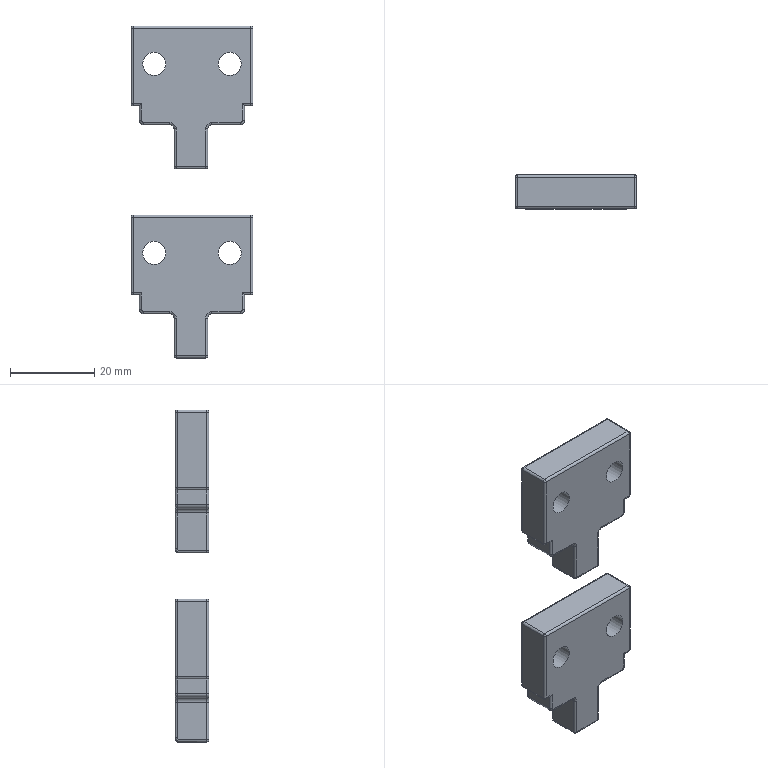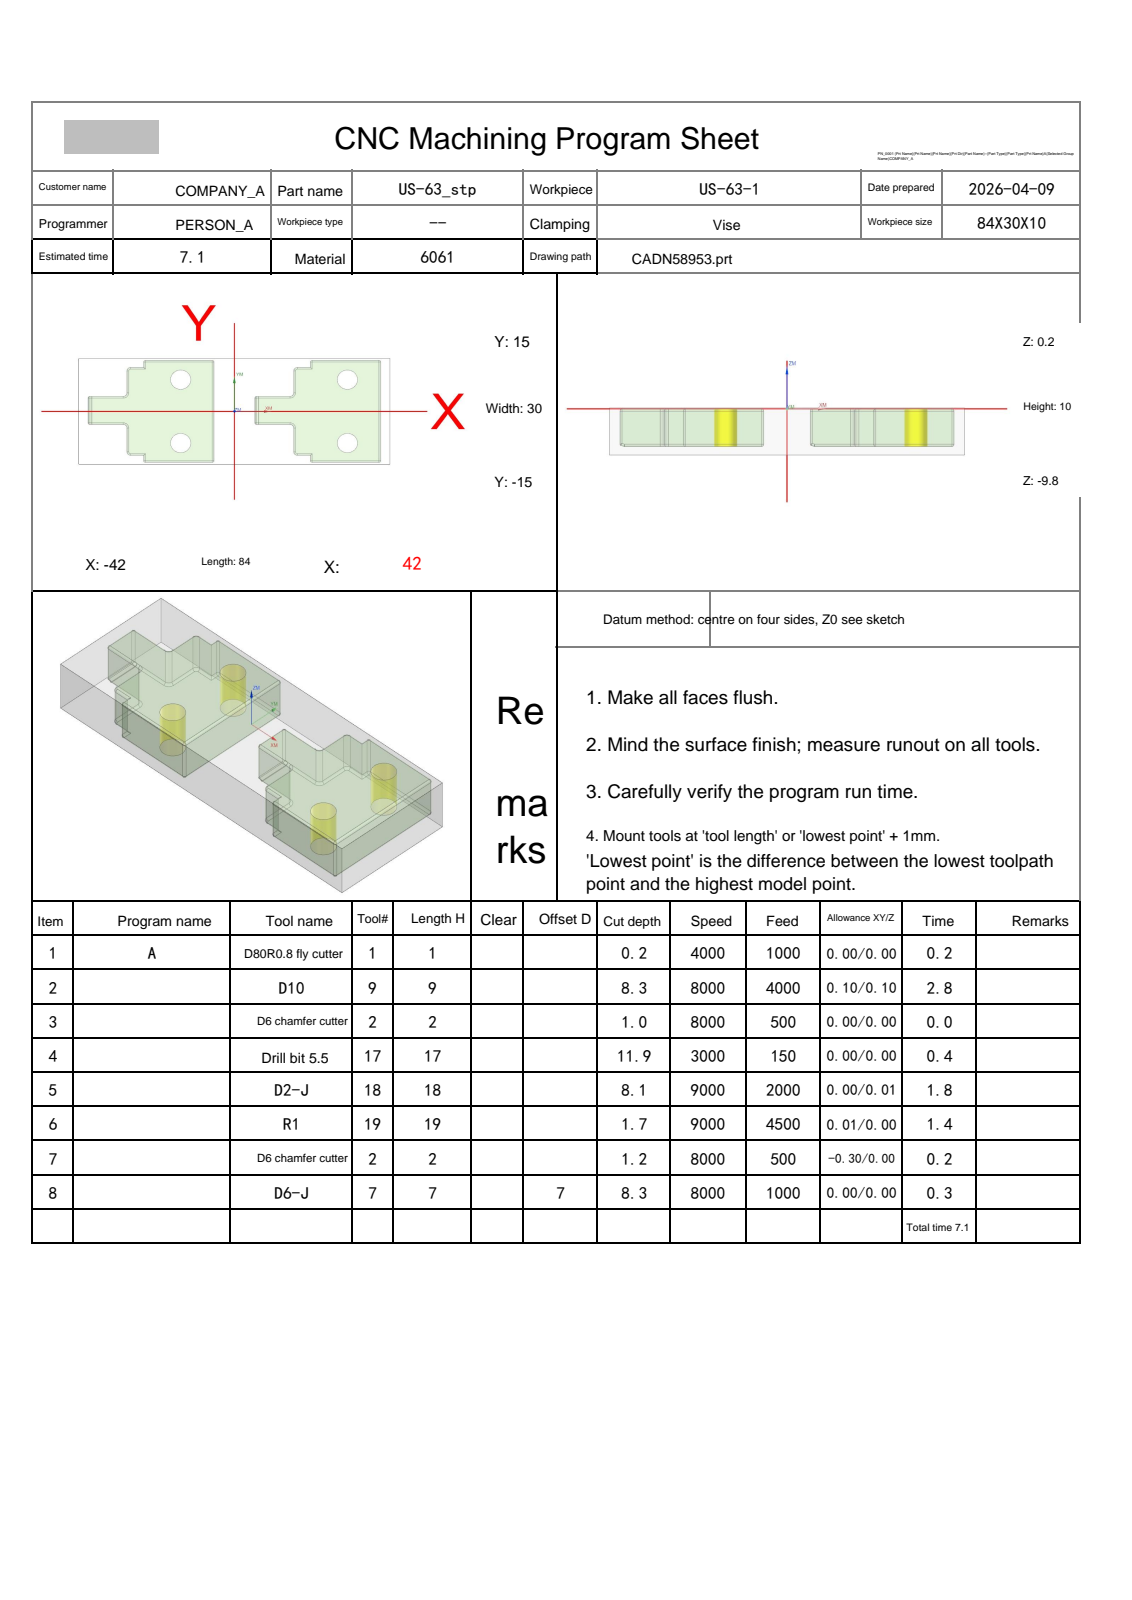NC program | NX | posted by the shop | part box 29 x 8 x 79 mm
Lines 1 to 33 of 24039:
%
O0001
(Machine time: 8.62 MIN)
(===Total Tool:7===)
(T1=D80R0.8 fly cutter D=80.  R=0.8  D-  H01 Z=0.    )
(T9=D10     D=10.  R=0.   D-  H09 Z=-8.1  )
(T2=D6 chamfer cutter   D=6.   R=0.   D-  H02 Z=-1.   )
(T17=Drill bit 5.5  D=5.5  DR_a=118 D-  H17 Z=-11.65)
(T18=D2-J   D=2.   R=0.   D-  H18 Z=-7.95 )
(T19=R1     D=2.   R=1.   D-  H19 Z=-1.5  )
(T7=D6-J    D=6.   R=0.   D7  H07 Z=-8.1  )
G80 G90 G17 G49 G40
G91 G28 Z0
M01
N1 T01 M06
(D80R0.8 fly cutter  D=80. R=0.8 H=01 ce=0.00 di=0.00)
G00 G90 G54 X-84.5 Y0.0 M03 S4000
G43 H01 Z20.
M08
Z2.
G01 Z0.0 F1000.
X-79.5
X79.5
X84.5
Z2.
G00 Z20.
G91 G28 Z0.0
M05
M09
G91 G28 Z0.0
M01